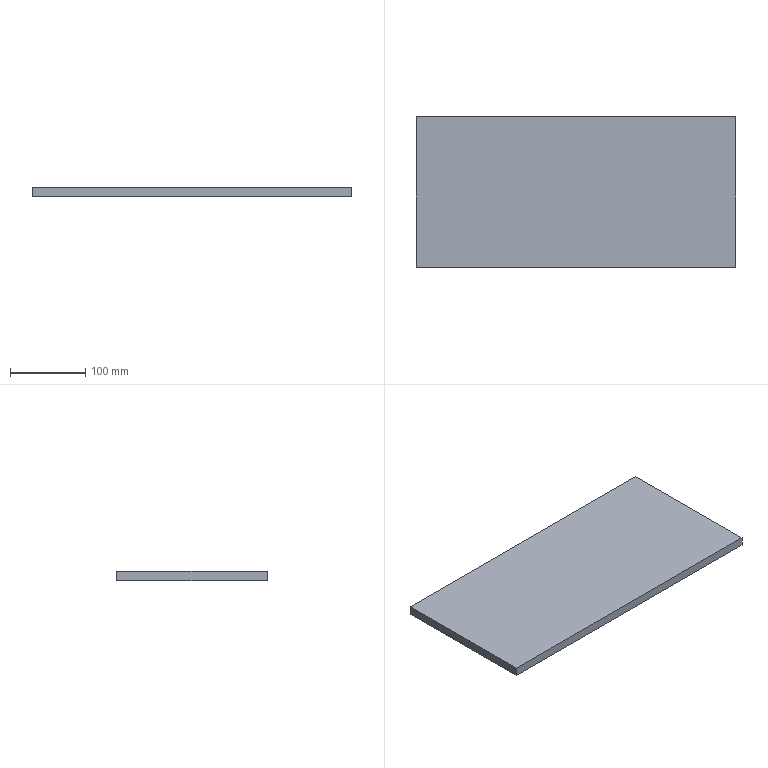Part | SolidWorks | features Extrusion 1 | 1 solid | 6 faces | box 425 x 200 x 12 mm | volume 1020000 mm3 | plane 6
STEP:
#1=CARTESIAN_POINT('',(0.,200.,0.));
#2=VERTEX_POINT('',#1);
#3=CARTESIAN_POINT('',(0.,0.,0.));
#4=VERTEX_POINT('',#3);
#5=CARTESIAN_POINT('',(0.,0.,0.));
#6=DIRECTION('',(0.,-1.,0.));
#7=VECTOR('',#6,1000.);
#8=LINE('',#5,#7);
#9=EDGE_CURVE('',#2,#4,#8,.T.);
#10=ORIENTED_EDGE('',*,*,#9,.T.);
#11=CARTESIAN_POINT('',(0.,0.,12.));
#12=VERTEX_POINT('',#11);
#13=CARTESIAN_POINT('',(0.,0.,12.));
#14=DIRECTION('',(0.,0.,-1.));
#15=VECTOR('',#14,1000.);
#16=LINE('',#13,#15);
#17=EDGE_CURVE('',#12,#4,#16,.T.);
#18=ORIENTED_EDGE('',*,*,#17,.F.);
#19=CARTESIAN_POINT('',(0.,200.,12.));
#20=VERTEX_POINT('',#19);
#21=CARTESIAN_POINT('',(0.,0.,12.));
#22=DIRECTION('',(0.,-1.,0.));
#23=VECTOR('',#22,1000.);
#24=LINE('',#21,#23);
#25=EDGE_CURVE('',#20,#12,#24,.T.);
#26=ORIENTED_EDGE('',*,*,#25,.F.);
#27=CARTESIAN_POINT('',(0.,200.,12.));
#28=DIRECTION('',(0.,0.,-1.));
#29=VECTOR('',#28,1000.);
#30=LINE('',#27,#29);
#31=EDGE_CURVE('',#20,#2,#30,.T.);
#32=ORIENTED_EDGE('',*,*,#31,.T.);
#33=EDGE_LOOP('',(#10,#18,#26,#32));
#34=FACE_OUTER_BOUND('',#33,.T.);
#35=CARTESIAN_POINT('',(0.,0.,12.));
#36=DIRECTION('',(1.,0.,0.));
#37=DIRECTION('',(0.,0.,-1.));
#38=AXIS2_PLACEMENT_3D('',#35,#36,#37);
#39=PLANE('',#38);
#40=ADVANCED_FACE('',(#34),#39,.F.);
#41=CARTESIAN_POINT('',(425.,0.,0.));
#42=VERTEX_POINT('',#41);
#43=CARTESIAN_POINT('',(0.,0.,0.));
#44=DIRECTION('',(1.,0.,0.));
#45=VECTOR('',#44,1000.);
#46=LINE('',#43,#45);
#47=EDGE_CURVE('',#4,#42,#46,.T.);
#48=ORIENTED_EDGE('',*,*,#47,.T.);
#49=CARTESIAN_POINT('',(425.,0.,12.));
#50=VERTEX_POINT('',#49);
#51=CARTESIAN_POINT('',(425.,0.,12.));
#52=DIRECTION('',(0.,0.,-1.));
#53=VECTOR('',#52,1000.);
#54=LINE('',#51,#53);
#55=EDGE_CURVE('',#50,#42,#54,.T.);
#56=ORIENTED_EDGE('',*,*,#55,.F.);
#57=CARTESIAN_POINT('',(0.,0.,12.));
#58=DIRECTION('',(1.,0.,0.));
#59=VECTOR('',#58,1000.);
#60=LINE('',#57,#59);
#61=EDGE_CURVE('',#12,#50,#60,.T.);
#62=ORIENTED_EDGE('',*,*,#61,.F.);
#63=ORIENTED_EDGE('',*,*,#17,.T.);
#64=EDGE_LOOP('',(#48,#56,#62,#63));
#65=FACE_OUTER_BOUND('',#64,.T.);
#66=CARTESIAN_POINT('',(0.,0.,12.));
#67=DIRECTION('',(0.,1.,0.));
#68=DIRECTION('',(0.,0.,1.));
#69=AXIS2_PLACEMENT_3D('',#66,#67,#68);
#70=PLANE('',#69);
#71=ADVANCED_FACE('',(#65),#70,.F.);
#72=CARTESIAN_POINT('',(425.,200.,0.));
#73=VERTEX_POINT('',#72);
#74=CARTESIAN_POINT('',(425.,0.,0.));
#75=DIRECTION('',(0.,1.,0.));
#76=VECTOR('',#75,1000.);
#77=LINE('',#74,#76);
#78=EDGE_CURVE('',#42,#73,#77,.T.);
#79=ORIENTED_EDGE('',*,*,#78,.T.);
#80=CARTESIAN_POINT('',(425.,200.,12.));
#81=VERTEX_POINT('',#80);
#82=CARTESIAN_POINT('',(425.,200.,12.));
#83=DIRECTION('',(0.,0.,-1.));
#84=VECTOR('',#83,1000.);
#85=LINE('',#82,#84);
#86=EDGE_CURVE('',#81,#73,#85,.T.);
#87=ORIENTED_EDGE('',*,*,#86,.F.);
#88=CARTESIAN_POINT('',(425.,0.,12.));
#89=DIRECTION('',(0.,1.,0.));
#90=VECTOR('',#89,1000.);
#91=LINE('',#88,#90);
#92=EDGE_CURVE('',#50,#81,#91,.T.);
#93=ORIENTED_EDGE('',*,*,#92,.F.);
#94=ORIENTED_EDGE('',*,*,#55,.T.);
#95=EDGE_LOOP('',(#79,#87,#93,#94));
#96=FACE_OUTER_BOUND('',#95,.T.);
#97=CARTESIAN_POINT('',(425.,0.,12.));
#98=DIRECTION('',(-1.,0.,0.));
#99=DIRECTION('',(0.,0.,1.));
#100=AXIS2_PLACEMENT_3D('',#97,#98,#99);
#101=PLANE('',#100);
#102=ADVANCED_FACE('',(#96),#101,.F.);
#103=CARTESIAN_POINT('',(0.,200.,0.));
#104=DIRECTION('',(-1.,0.,0.));
#105=VECTOR('',#104,1000.);
#106=LINE('',#103,#105);
#107=EDGE_CURVE('',#73,#2,#106,.T.);
#108=ORIENTED_EDGE('',*,*,#107,.T.);
#109=ORIENTED_EDGE('',*,*,#31,.F.);
#110=CARTESIAN_POINT('',(0.,200.,12.));
#111=DIRECTION('',(-1.,0.,0.));
#112=VECTOR('',#111,1000.);
#113=LINE('',#110,#112);
#114=EDGE_CURVE('',#81,#20,#113,.T.);
#115=ORIENTED_EDGE('',*,*,#114,.F.);
#116=ORIENTED_EDGE('',*,*,#86,.T.);
#117=EDGE_LOOP('',(#108,#109,#115,#116));
#118=FACE_OUTER_BOUND('',#117,.T.);
#119=CARTESIAN_POINT('',(0.,200.,12.));
#120=DIRECTION('',(0.,-1.,0.));
#121=DIRECTION('',(0.,0.,-1.));
#122=AXIS2_PLACEMENT_3D('',#119,#120,#121);
#123=PLANE('',#122);
#124=ADVANCED_FACE('',(#118),#123,.F.);
#125=ORIENTED_EDGE('',*,*,#25,.T.);
#126=ORIENTED_EDGE('',*,*,#61,.T.);
#127=ORIENTED_EDGE('',*,*,#92,.T.);
#128=ORIENTED_EDGE('',*,*,#114,.T.);
#129=EDGE_LOOP('',(#125,#126,#127,#128));
#130=FACE_OUTER_BOUND('',#129,.T.);
#131=CARTESIAN_POINT('',(0.,0.,12.));
#132=DIRECTION('',(0.,0.,-1.));
#133=DIRECTION('',(-1.,0.,0.));
#134=AXIS2_PLACEMENT_3D('',#131,#132,#133);
#135=PLANE('',#134);
#136=ADVANCED_FACE('',(#130),#135,.F.);
#137=ORIENTED_EDGE('',*,*,#9,.F.);
#138=ORIENTED_EDGE('',*,*,#107,.F.);
#139=ORIENTED_EDGE('',*,*,#78,.F.);
#140=ORIENTED_EDGE('',*,*,#47,.F.);
#141=EDGE_LOOP('',(#137,#138,#139,#140));
#142=FACE_OUTER_BOUND('',#141,.T.);
#143=CARTESIAN_POINT('',(0.,0.,0.));
#144=DIRECTION('',(0.,0.,-1.));
#145=DIRECTION('',(-1.,0.,0.));
#146=AXIS2_PLACEMENT_3D('',#143,#144,#145);
#147=PLANE('',#146);
#148=ADVANCED_FACE('',(#142),#147,.T.);
#149=CLOSED_SHELL('',(#40,#71,#102,#124,#136,#148));
#150=MANIFOLD_SOLID_BREP('',#149);
#151=CARTESIAN_POINT('',(0.,0.,0.));
#152=DIRECTION('',(0.,0.,1.));
#153=DIRECTION('',(1.,0.,0.));
#154=AXIS2_PLACEMENT_3D('',#151,#152,#153);
#155=(LENGTH_UNIT()NAMED_UNIT(*)SI_UNIT(.MILLI.,.METRE.));
#156=UNCERTAINTY_MEASURE_WITH_UNIT(LENGTH_MEASURE(0.00001),#155,'','');
#157=(NAMED_UNIT(*)PLANE_ANGLE_UNIT()SI_UNIT($,.RADIAN.));
#158=(NAMED_UNIT(*)SI_UNIT($,.STERADIAN.)SOLID_ANGLE_UNIT());
#159=(GEOMETRIC_REPRESENTATION_CONTEXT(3)GLOBAL_UNCERTAINTY_ASSIGNED_CONTEXT((#156))GLOBAL_UNIT_ASSIGNED_CONTEXT((#155,#157,#158))REPRESENTATION_CONTEXT('',''));
#160=ADVANCED_BREP_SHAPE_REPRESENTATION('',(#150,#154),#159);